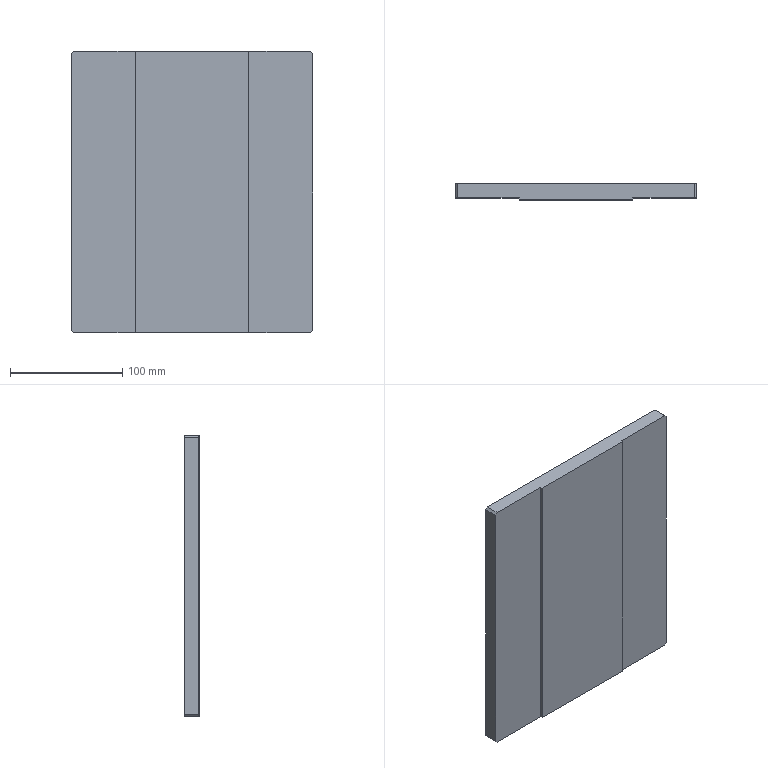Part | SolidWorks | features ICE 2, Chamfer 1, Extrusion 1, Fillet 1 | 1 solid | 14 faces | box 215 x 14 x 250 mm | volume 709650 mm3 | plane 14
STEP:
#1=CARTESIAN_POINT('',(107.5,-5.5,-123.));
#2=VERTEX_POINT('',#1);
#3=CARTESIAN_POINT('',(107.5,-5.5,123.));
#4=VERTEX_POINT('',#3);
#5=CARTESIAN_POINT('',(107.5,-5.5,-125.));
#6=DIRECTION('',(0.,0.,1.));
#7=VECTOR('',#6,1000.);
#8=LINE('',#5,#7);
#9=EDGE_CURVE('',#2,#4,#8,.T.);
#10=ORIENTED_EDGE('',*,*,#9,.F.);
#11=CARTESIAN_POINT('',(107.5,7.,-123.));
#12=VERTEX_POINT('',#11);
#13=CARTESIAN_POINT('',(107.5,7.,-123.));
#14=DIRECTION('',(0.,1.,0.));
#15=VECTOR('',#14,1000.);
#16=LINE('',#13,#15);
#17=EDGE_CURVE('',#2,#12,#16,.T.);
#18=ORIENTED_EDGE('',*,*,#17,.T.);
#19=CARTESIAN_POINT('',(107.5,7.,123.));
#20=VERTEX_POINT('',#19);
#21=CARTESIAN_POINT('',(107.5,7.,125.));
#22=DIRECTION('',(0.,0.,-1.));
#23=VECTOR('',#22,1000.);
#24=LINE('',#21,#23);
#25=EDGE_CURVE('',#20,#12,#24,.T.);
#26=ORIENTED_EDGE('',*,*,#25,.F.);
#27=CARTESIAN_POINT('',(107.5,7.,123.));
#28=DIRECTION('',(0.,-1.,0.));
#29=VECTOR('',#28,1000.);
#30=LINE('',#27,#29);
#31=EDGE_CURVE('',#20,#4,#30,.T.);
#32=ORIENTED_EDGE('',*,*,#31,.T.);
#33=EDGE_LOOP('',(#10,#18,#26,#32));
#34=FACE_OUTER_BOUND('',#33,.T.);
#35=CARTESIAN_POINT('',(107.5,7.,125.));
#36=DIRECTION('',(-1.,0.,0.));
#37=DIRECTION('',(0.,0.,1.));
#38=AXIS2_PLACEMENT_3D('',#35,#36,#37);
#39=PLANE('',#38);
#40=ADVANCED_FACE('',(#34),#39,.F.);
#41=CARTESIAN_POINT('',(105.5,7.,-125.));
#42=VERTEX_POINT('',#41);
#43=CARTESIAN_POINT('',(-105.5,7.,-125.));
#44=VERTEX_POINT('',#43);
#45=CARTESIAN_POINT('',(-107.5,7.,-125.));
#46=DIRECTION('',(-1.,0.,0.));
#47=VECTOR('',#46,1000.);
#48=LINE('',#45,#47);
#49=EDGE_CURVE('',#42,#44,#48,.T.);
#50=ORIENTED_EDGE('',*,*,#49,.F.);
#51=CARTESIAN_POINT('',(105.5,-5.5,-125.));
#52=VERTEX_POINT('',#51);
#53=CARTESIAN_POINT('',(105.5,7.,-125.));
#54=DIRECTION('',(0.,-1.,0.));
#55=VECTOR('',#54,1000.);
#56=LINE('',#53,#55);
#57=EDGE_CURVE('',#42,#52,#56,.T.);
#58=ORIENTED_EDGE('',*,*,#57,.T.);
#59=CARTESIAN_POINT('',(50.5,-5.5,-125.));
#60=VERTEX_POINT('',#59);
#61=CARTESIAN_POINT('',(107.5,-5.5,-125.));
#62=DIRECTION('',(1.,0.,0.));
#63=VECTOR('',#62,1000.);
#64=LINE('',#61,#63);
#65=EDGE_CURVE('',#60,#52,#64,.T.);
#66=ORIENTED_EDGE('',*,*,#65,.F.);
#67=CARTESIAN_POINT('',(50.5,-7.,-125.));
#68=VERTEX_POINT('',#67);
#69=CARTESIAN_POINT('',(50.5,-5.5,-125.));
#70=DIRECTION('',(0.,-1.,0.));
#71=VECTOR('',#70,1000.);
#72=LINE('',#69,#71);
#73=EDGE_CURVE('',#60,#68,#72,.T.);
#74=ORIENTED_EDGE('',*,*,#73,.T.);
#75=CARTESIAN_POINT('',(-50.5,-7.,-125.));
#76=VERTEX_POINT('',#75);
#77=CARTESIAN_POINT('',(-107.5,-7.,-125.));
#78=DIRECTION('',(-1.,0.,0.));
#79=VECTOR('',#78,1000.);
#80=LINE('',#77,#79);
#81=EDGE_CURVE('',#68,#76,#80,.T.);
#82=ORIENTED_EDGE('',*,*,#81,.T.);
#83=CARTESIAN_POINT('',(-50.5,-5.5,-125.));
#84=VERTEX_POINT('',#83);
#85=CARTESIAN_POINT('',(-50.5,-5.5,-125.));
#86=DIRECTION('',(0.,-1.,0.));
#87=VECTOR('',#86,1000.);
#88=LINE('',#85,#87);
#89=EDGE_CURVE('',#84,#76,#88,.T.);
#90=ORIENTED_EDGE('',*,*,#89,.F.);
#91=CARTESIAN_POINT('',(-105.5,-5.5,-125.));
#92=VERTEX_POINT('',#91);
#93=CARTESIAN_POINT('',(-107.5,-5.5,-125.));
#94=DIRECTION('',(1.,0.,0.));
#95=VECTOR('',#94,1000.);
#96=LINE('',#93,#95);
#97=EDGE_CURVE('',#92,#84,#96,.T.);
#98=ORIENTED_EDGE('',*,*,#97,.F.);
#99=CARTESIAN_POINT('',(-105.5,7.,-125.));
#100=DIRECTION('',(0.,1.,0.));
#101=VECTOR('',#100,1000.);
#102=LINE('',#99,#101);
#103=EDGE_CURVE('',#92,#44,#102,.T.);
#104=ORIENTED_EDGE('',*,*,#103,.T.);
#105=EDGE_LOOP('',(#50,#58,#66,#74,#82,#90,#98,#104));
#106=FACE_OUTER_BOUND('',#105,.T.);
#107=CARTESIAN_POINT('',(-107.5,7.,-125.));
#108=DIRECTION('',(0.,0.,1.));
#109=DIRECTION('',(1.,0.,0.));
#110=AXIS2_PLACEMENT_3D('',#107,#108,#109);
#111=PLANE('',#110);
#112=ADVANCED_FACE('',(#106),#111,.F.);
#113=CARTESIAN_POINT('',(-107.5,7.,-123.));
#114=VERTEX_POINT('',#113);
#115=CARTESIAN_POINT('',(-107.5,7.,123.));
#116=VERTEX_POINT('',#115);
#117=CARTESIAN_POINT('',(-107.5,7.,125.));
#118=DIRECTION('',(0.,0.,1.));
#119=VECTOR('',#118,1000.);
#120=LINE('',#117,#119);
#121=EDGE_CURVE('',#114,#116,#120,.T.);
#122=ORIENTED_EDGE('',*,*,#121,.F.);
#123=CARTESIAN_POINT('',(-107.5,-5.5,-123.));
#124=VERTEX_POINT('',#123);
#125=CARTESIAN_POINT('',(-107.5,7.,-123.));
#126=DIRECTION('',(0.,-1.,0.));
#127=VECTOR('',#126,1000.);
#128=LINE('',#125,#127);
#129=EDGE_CURVE('',#114,#124,#128,.T.);
#130=ORIENTED_EDGE('',*,*,#129,.T.);
#131=CARTESIAN_POINT('',(-107.5,-5.5,123.));
#132=VERTEX_POINT('',#131);
#133=CARTESIAN_POINT('',(-107.5,-5.5,-125.));
#134=DIRECTION('',(0.,0.,-1.));
#135=VECTOR('',#134,1000.);
#136=LINE('',#133,#135);
#137=EDGE_CURVE('',#132,#124,#136,.T.);
#138=ORIENTED_EDGE('',*,*,#137,.F.);
#139=CARTESIAN_POINT('',(-107.5,7.,123.));
#140=DIRECTION('',(0.,1.,0.));
#141=VECTOR('',#140,1000.);
#142=LINE('',#139,#141);
#143=EDGE_CURVE('',#132,#116,#142,.T.);
#144=ORIENTED_EDGE('',*,*,#143,.T.);
#145=EDGE_LOOP('',(#122,#130,#138,#144));
#146=FACE_OUTER_BOUND('',#145,.T.);
#147=CARTESIAN_POINT('',(-107.5,7.,125.));
#148=DIRECTION('',(1.,0.,0.));
#149=DIRECTION('',(0.,0.,-1.));
#150=AXIS2_PLACEMENT_3D('',#147,#148,#149);
#151=PLANE('',#150);
#152=ADVANCED_FACE('',(#146),#151,.F.);
#153=CARTESIAN_POINT('',(-105.5,7.,125.));
#154=VERTEX_POINT('',#153);
#155=CARTESIAN_POINT('',(105.5,7.,125.));
#156=VERTEX_POINT('',#155);
#157=CARTESIAN_POINT('',(-107.5,7.,125.));
#158=DIRECTION('',(1.,0.,0.));
#159=VECTOR('',#158,1000.);
#160=LINE('',#157,#159);
#161=EDGE_CURVE('',#154,#156,#160,.T.);
#162=ORIENTED_EDGE('',*,*,#161,.F.);
#163=CARTESIAN_POINT('',(-105.5,-5.5,125.));
#164=VERTEX_POINT('',#163);
#165=CARTESIAN_POINT('',(-105.5,7.,125.));
#166=DIRECTION('',(0.,-1.,0.));
#167=VECTOR('',#166,1000.);
#168=LINE('',#165,#167);
#169=EDGE_CURVE('',#154,#164,#168,.T.);
#170=ORIENTED_EDGE('',*,*,#169,.T.);
#171=CARTESIAN_POINT('',(-50.5,-5.5,125.));
#172=VERTEX_POINT('',#171);
#173=CARTESIAN_POINT('',(-107.5,-5.5,125.));
#174=DIRECTION('',(-1.,0.,0.));
#175=VECTOR('',#174,1000.);
#176=LINE('',#173,#175);
#177=EDGE_CURVE('',#172,#164,#176,.T.);
#178=ORIENTED_EDGE('',*,*,#177,.F.);
#179=CARTESIAN_POINT('',(-50.5,-7.,125.));
#180=VERTEX_POINT('',#179);
#181=CARTESIAN_POINT('',(-50.5,-5.5,125.));
#182=DIRECTION('',(0.,-1.,0.));
#183=VECTOR('',#182,1000.);
#184=LINE('',#181,#183);
#185=EDGE_CURVE('',#172,#180,#184,.T.);
#186=ORIENTED_EDGE('',*,*,#185,.T.);
#187=CARTESIAN_POINT('',(50.5,-7.,125.));
#188=VERTEX_POINT('',#187);
#189=CARTESIAN_POINT('',(-107.5,-7.,125.));
#190=DIRECTION('',(1.,0.,0.));
#191=VECTOR('',#190,1000.);
#192=LINE('',#189,#191);
#193=EDGE_CURVE('',#180,#188,#192,.T.);
#194=ORIENTED_EDGE('',*,*,#193,.T.);
#195=CARTESIAN_POINT('',(50.5,-5.5,125.));
#196=VERTEX_POINT('',#195);
#197=CARTESIAN_POINT('',(50.5,-5.5,125.));
#198=DIRECTION('',(0.,-1.,0.));
#199=VECTOR('',#198,1000.);
#200=LINE('',#197,#199);
#201=EDGE_CURVE('',#196,#188,#200,.T.);
#202=ORIENTED_EDGE('',*,*,#201,.F.);
#203=CARTESIAN_POINT('',(105.5,-5.5,125.));
#204=VERTEX_POINT('',#203);
#205=CARTESIAN_POINT('',(107.5,-5.5,125.));
#206=DIRECTION('',(-1.,0.,0.));
#207=VECTOR('',#206,1000.);
#208=LINE('',#205,#207);
#209=EDGE_CURVE('',#204,#196,#208,.T.);
#210=ORIENTED_EDGE('',*,*,#209,.F.);
#211=CARTESIAN_POINT('',(105.5,7.,125.));
#212=DIRECTION('',(0.,1.,0.));
#213=VECTOR('',#212,1000.);
#214=LINE('',#211,#213);
#215=EDGE_CURVE('',#204,#156,#214,.T.);
#216=ORIENTED_EDGE('',*,*,#215,.T.);
#217=EDGE_LOOP('',(#162,#170,#178,#186,#194,#202,#210,#216));
#218=FACE_OUTER_BOUND('',#217,.T.);
#219=CARTESIAN_POINT('',(-107.5,7.,125.));
#220=DIRECTION('',(0.,0.,-1.));
#221=DIRECTION('',(-1.,0.,0.));
#222=AXIS2_PLACEMENT_3D('',#219,#220,#221);
#223=PLANE('',#222);
#224=ADVANCED_FACE('',(#218),#223,.F.);
#225=ORIENTED_EDGE('',*,*,#25,.T.);
#226=CARTESIAN_POINT('',(105.5,7.,-125.));
#227=DIRECTION('',(-0.7071,0.,-0.7071));
#228=VECTOR('',#227,1000.);
#229=LINE('',#226,#228);
#230=EDGE_CURVE('',#12,#42,#229,.T.);
#231=ORIENTED_EDGE('',*,*,#230,.T.);
#232=ORIENTED_EDGE('',*,*,#49,.T.);
#233=CARTESIAN_POINT('',(-107.5,7.,-123.));
#234=DIRECTION('',(-0.7071,0.,0.7071));
#235=VECTOR('',#234,1000.);
#236=LINE('',#233,#235);
#237=EDGE_CURVE('',#44,#114,#236,.T.);
#238=ORIENTED_EDGE('',*,*,#237,.T.);
#239=ORIENTED_EDGE('',*,*,#121,.T.);
#240=CARTESIAN_POINT('',(-105.5,7.,125.));
#241=DIRECTION('',(0.7071,0.,0.7071));
#242=VECTOR('',#241,1000.);
#243=LINE('',#240,#242);
#244=EDGE_CURVE('',#116,#154,#243,.T.);
#245=ORIENTED_EDGE('',*,*,#244,.T.);
#246=ORIENTED_EDGE('',*,*,#161,.T.);
#247=CARTESIAN_POINT('',(107.5,7.,123.));
#248=DIRECTION('',(0.7071,0.,-0.7071));
#249=VECTOR('',#248,1000.);
#250=LINE('',#247,#249);
#251=EDGE_CURVE('',#156,#20,#250,.T.);
#252=ORIENTED_EDGE('',*,*,#251,.T.);
#253=EDGE_LOOP('',(#225,#231,#232,#238,#239,#245,#246,#252));
#254=FACE_OUTER_BOUND('',#253,.T.);
#255=CARTESIAN_POINT('',(0.,7.,0.));
#256=DIRECTION('',(0.,-1.,0.));
#257=DIRECTION('',(0.,0.,-1.));
#258=AXIS2_PLACEMENT_3D('',#255,#256,#257);
#259=PLANE('',#258);
#260=ADVANCED_FACE('',(#254),#259,.F.);
#261=CARTESIAN_POINT('',(50.5,-7.,-125.));
#262=DIRECTION('',(0.,0.,-1.));
#263=VECTOR('',#262,1000.);
#264=LINE('',#261,#263);
#265=EDGE_CURVE('',#188,#68,#264,.T.);
#266=ORIENTED_EDGE('',*,*,#265,.F.);
#267=ORIENTED_EDGE('',*,*,#193,.F.);
#268=CARTESIAN_POINT('',(-50.5,-7.,-125.));
#269=DIRECTION('',(0.,0.,1.));
#270=VECTOR('',#269,1000.);
#271=LINE('',#268,#270);
#272=EDGE_CURVE('',#76,#180,#271,.T.);
#273=ORIENTED_EDGE('',*,*,#272,.F.);
#274=ORIENTED_EDGE('',*,*,#81,.F.);
#275=EDGE_LOOP('',(#266,#267,#273,#274));
#276=FACE_OUTER_BOUND('',#275,.T.);
#277=CARTESIAN_POINT('',(0.,-7.,0.));
#278=DIRECTION('',(0.,-1.,0.));
#279=DIRECTION('',(0.,0.,-1.));
#280=AXIS2_PLACEMENT_3D('',#277,#278,#279);
#281=PLANE('',#280);
#282=ADVANCED_FACE('',(#276),#281,.T.);
#283=ORIENTED_EDGE('',*,*,#272,.T.);
#284=ORIENTED_EDGE('',*,*,#185,.F.);
#285=CARTESIAN_POINT('',(-50.5,-5.5,-125.));
#286=DIRECTION('',(0.,0.,1.));
#287=VECTOR('',#286,1000.);
#288=LINE('',#285,#287);
#289=EDGE_CURVE('',#84,#172,#288,.T.);
#290=ORIENTED_EDGE('',*,*,#289,.F.);
#291=ORIENTED_EDGE('',*,*,#89,.T.);
#292=EDGE_LOOP('',(#283,#284,#290,#291));
#293=FACE_OUTER_BOUND('',#292,.T.);
#294=CARTESIAN_POINT('',(-50.5,-5.5,-125.));
#295=DIRECTION('',(1.,0.,0.));
#296=DIRECTION('',(0.,0.,-1.));
#297=AXIS2_PLACEMENT_3D('',#294,#295,#296);
#298=PLANE('',#297);
#299=ADVANCED_FACE('',(#293),#298,.F.);
#300=ORIENTED_EDGE('',*,*,#137,.T.);
#301=CARTESIAN_POINT('',(-107.5,-5.5,-123.));
#302=DIRECTION('',(0.7071,0.,-0.7071));
#303=VECTOR('',#302,1000.);
#304=LINE('',#301,#303);
#305=EDGE_CURVE('',#124,#92,#304,.T.);
#306=ORIENTED_EDGE('',*,*,#305,.T.);
#307=ORIENTED_EDGE('',*,*,#97,.T.);
#308=ORIENTED_EDGE('',*,*,#289,.T.);
#309=ORIENTED_EDGE('',*,*,#177,.T.);
#310=CARTESIAN_POINT('',(-105.5,-5.5,125.));
#311=DIRECTION('',(-0.7071,0.,-0.7071));
#312=VECTOR('',#311,1000.);
#313=LINE('',#310,#312);
#314=EDGE_CURVE('',#164,#132,#313,.T.);
#315=ORIENTED_EDGE('',*,*,#314,.T.);
#316=EDGE_LOOP('',(#300,#306,#307,#308,#309,#315));
#317=FACE_OUTER_BOUND('',#316,.T.);
#318=CARTESIAN_POINT('',(0.,-5.5,0.));
#319=DIRECTION('',(0.,1.,0.));
#320=DIRECTION('',(0.,0.,1.));
#321=AXIS2_PLACEMENT_3D('',#318,#319,#320);
#322=PLANE('',#321);
#323=ADVANCED_FACE('',(#317),#322,.F.);
#324=ORIENTED_EDGE('',*,*,#265,.T.);
#325=ORIENTED_EDGE('',*,*,#73,.F.);
#326=CARTESIAN_POINT('',(50.5,-5.5,-125.));
#327=DIRECTION('',(0.,0.,-1.));
#328=VECTOR('',#327,1000.);
#329=LINE('',#326,#328);
#330=EDGE_CURVE('',#196,#60,#329,.T.);
#331=ORIENTED_EDGE('',*,*,#330,.F.);
#332=ORIENTED_EDGE('',*,*,#201,.T.);
#333=EDGE_LOOP('',(#324,#325,#331,#332));
#334=FACE_OUTER_BOUND('',#333,.T.);
#335=CARTESIAN_POINT('',(50.5,-5.5,-125.));
#336=DIRECTION('',(-1.,0.,0.));
#337=DIRECTION('',(0.,0.,1.));
#338=AXIS2_PLACEMENT_3D('',#335,#336,#337);
#339=PLANE('',#338);
#340=ADVANCED_FACE('',(#334),#339,.F.);
#341=ORIENTED_EDGE('',*,*,#65,.T.);
#342=CARTESIAN_POINT('',(115.25,-5.5,-115.25));
#343=DIRECTION('',(0.7071,0.,0.7071));
#344=VECTOR('',#343,1000.);
#345=LINE('',#342,#344);
#346=EDGE_CURVE('',#52,#2,#345,.T.);
#347=ORIENTED_EDGE('',*,*,#346,.T.);
#348=ORIENTED_EDGE('',*,*,#9,.T.);
#349=CARTESIAN_POINT('',(115.25,-5.5,115.25));
#350=DIRECTION('',(-0.7071,0.,0.7071));
#351=VECTOR('',#350,1000.);
#352=LINE('',#349,#351);
#353=EDGE_CURVE('',#4,#204,#352,.T.);
#354=ORIENTED_EDGE('',*,*,#353,.T.);
#355=ORIENTED_EDGE('',*,*,#209,.T.);
#356=ORIENTED_EDGE('',*,*,#330,.T.);
#357=EDGE_LOOP('',(#341,#347,#348,#354,#355,#356));
#358=FACE_OUTER_BOUND('',#357,.T.);
#359=CARTESIAN_POINT('',(0.,-5.5,0.));
#360=DIRECTION('',(0.,-1.,0.));
#361=DIRECTION('',(0.,0.,-1.));
#362=AXIS2_PLACEMENT_3D('',#359,#360,#361);
#363=PLANE('',#362);
#364=ADVANCED_FACE('',(#358),#363,.T.);
#365=ORIENTED_EDGE('',*,*,#230,.F.);
#366=ORIENTED_EDGE('',*,*,#17,.F.);
#367=ORIENTED_EDGE('',*,*,#346,.F.);
#368=ORIENTED_EDGE('',*,*,#57,.F.);
#369=EDGE_LOOP('',(#365,#366,#367,#368));
#370=FACE_OUTER_BOUND('',#369,.T.);
#371=CARTESIAN_POINT('',(105.5,7.,-125.));
#372=DIRECTION('',(-0.7071,0.,0.7071));
#373=DIRECTION('',(0.,-1.,0.));
#374=AXIS2_PLACEMENT_3D('',#371,#372,#373);
#375=PLANE('',#374);
#376=ADVANCED_FACE('',(#370),#375,.F.);
#377=ORIENTED_EDGE('',*,*,#237,.F.);
#378=ORIENTED_EDGE('',*,*,#103,.F.);
#379=ORIENTED_EDGE('',*,*,#305,.F.);
#380=ORIENTED_EDGE('',*,*,#129,.F.);
#381=EDGE_LOOP('',(#377,#378,#379,#380));
#382=FACE_OUTER_BOUND('',#381,.T.);
#383=CARTESIAN_POINT('',(-107.5,7.,-123.));
#384=DIRECTION('',(0.7071,0.,0.7071));
#385=DIRECTION('',(0.,-1.,0.));
#386=AXIS2_PLACEMENT_3D('',#383,#384,#385);
#387=PLANE('',#386);
#388=ADVANCED_FACE('',(#382),#387,.F.);
#389=ORIENTED_EDGE('',*,*,#244,.F.);
#390=ORIENTED_EDGE('',*,*,#143,.F.);
#391=ORIENTED_EDGE('',*,*,#314,.F.);
#392=ORIENTED_EDGE('',*,*,#169,.F.);
#393=EDGE_LOOP('',(#389,#390,#391,#392));
#394=FACE_OUTER_BOUND('',#393,.T.);
#395=CARTESIAN_POINT('',(-105.5,7.,125.));
#396=DIRECTION('',(0.7071,0.,-0.7071));
#397=DIRECTION('',(0.,-1.,0.));
#398=AXIS2_PLACEMENT_3D('',#395,#396,#397);
#399=PLANE('',#398);
#400=ADVANCED_FACE('',(#394),#399,.F.);
#401=ORIENTED_EDGE('',*,*,#251,.F.);
#402=ORIENTED_EDGE('',*,*,#215,.F.);
#403=ORIENTED_EDGE('',*,*,#353,.F.);
#404=ORIENTED_EDGE('',*,*,#31,.F.);
#405=EDGE_LOOP('',(#401,#402,#403,#404));
#406=FACE_OUTER_BOUND('',#405,.T.);
#407=CARTESIAN_POINT('',(107.5,7.,123.));
#408=DIRECTION('',(-0.7071,0.,-0.7071));
#409=DIRECTION('',(0.,-1.,0.));
#410=AXIS2_PLACEMENT_3D('',#407,#408,#409);
#411=PLANE('',#410);
#412=ADVANCED_FACE('',(#406),#411,.F.);
#413=CLOSED_SHELL('',(#40,#112,#152,#224,#260,#282,#299,#323,#340,#364,#376,#388,#400,#412));
#414=MANIFOLD_SOLID_BREP('',#413);
#415=CARTESIAN_POINT('',(0.,0.,0.));
#416=DIRECTION('',(0.,0.,1.));
#417=DIRECTION('',(1.,0.,0.));
#418=AXIS2_PLACEMENT_3D('',#415,#416,#417);
#419=(LENGTH_UNIT()NAMED_UNIT(*)SI_UNIT(.MILLI.,.METRE.));
#420=UNCERTAINTY_MEASURE_WITH_UNIT(LENGTH_MEASURE(0.00001),#419,'','');
#421=(NAMED_UNIT(*)PLANE_ANGLE_UNIT()SI_UNIT($,.RADIAN.));
#422=(NAMED_UNIT(*)SI_UNIT($,.STERADIAN.)SOLID_ANGLE_UNIT());
#423=(GEOMETRIC_REPRESENTATION_CONTEXT(3)GLOBAL_UNCERTAINTY_ASSIGNED_CONTEXT((#420))GLOBAL_UNIT_ASSIGNED_CONTEXT((#419,#421,#422))REPRESENTATION_CONTEXT('',''));
#424=ADVANCED_BREP_SHAPE_REPRESENTATION('',(#414,#418),#423);